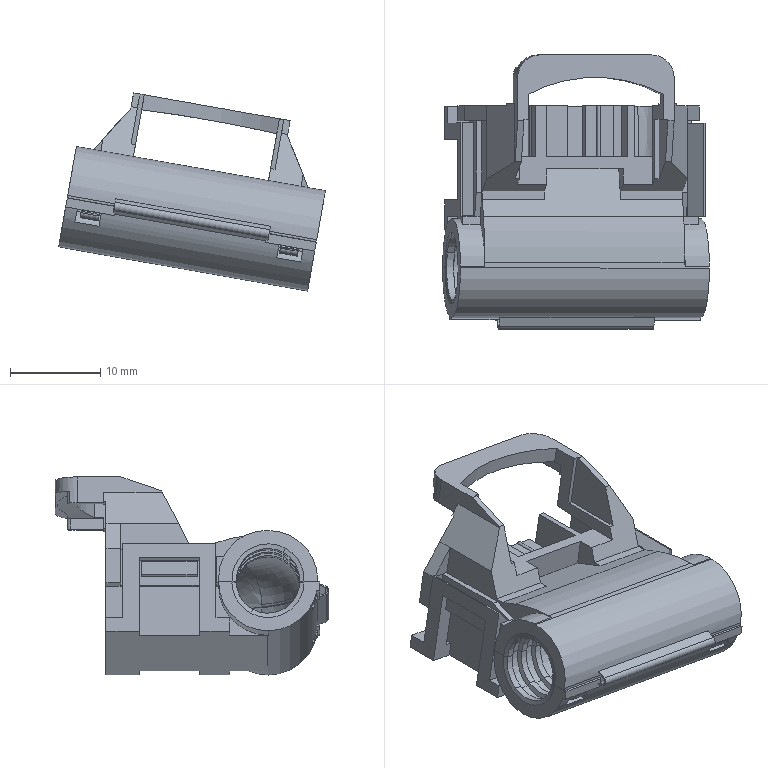Part | SolidWorks | features BaseBody 1 | 1 solid | 324 faces | box 29.543 x 30.33 x 21.946 mm | volume 3664 mm3 | plane 204 | cylinder 76 | cone 26 | spline 12 | torus 6 | commonest cylinder face diameters 8 x20 7 x12 0.6 x7 0.75 x6 11 x5 0.4 x3